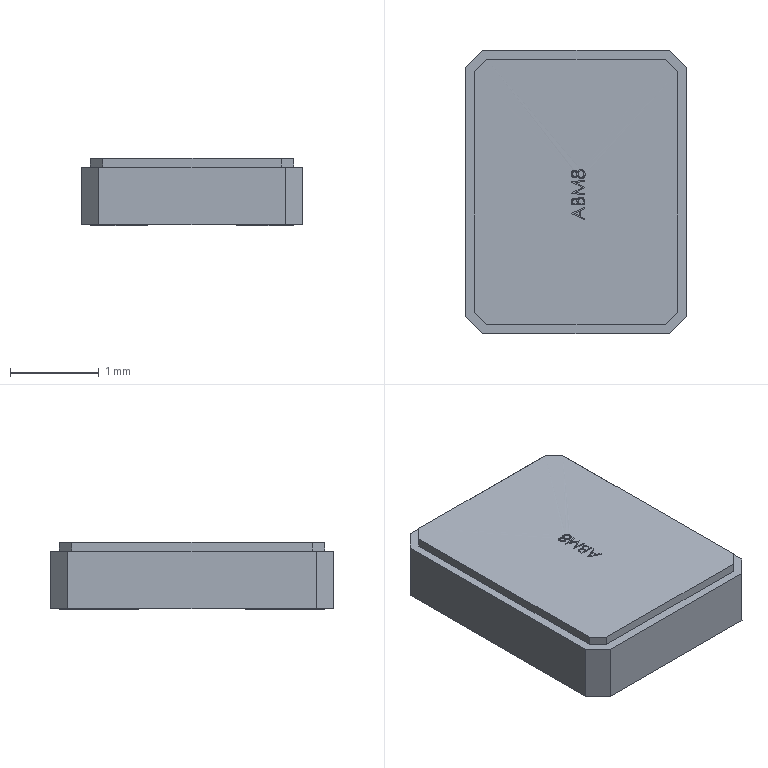Part | STEP file | RJ-USIO-V1_2-220411_79 | 1 solid | 112 faces | box 2.5 x 3.2 x 0.7611 mm | volume 5.856 mm3 | plane 86 | other 14 | cylinder 12 | commonest cylinder face diameters 0.093 x2 0.055 x1 0.056 x1 0.057 x1 0.069 x1 0.071 x1